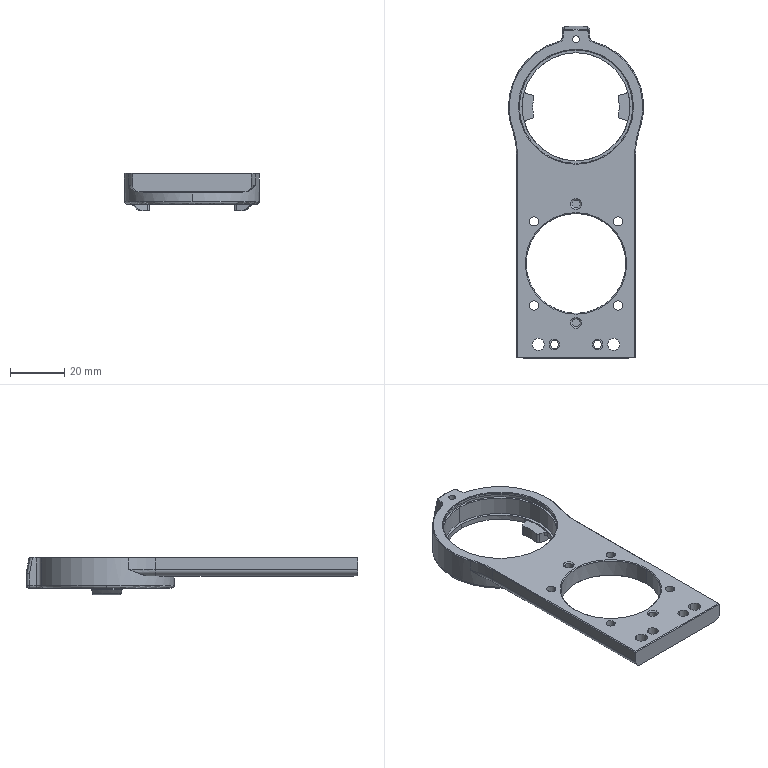NC program | NX | posted with a generic post | part box 50 x 122.9 x 14 mm
Lines 2916 to 3839 of 10876:
(ZLEVEL_PROFILE_1_COPY , TOOL : D3R0.5)
N5782 T18 M6
N5784 G54
N5786 G17 G0 G90 X85.63 Y20.139 S9500 M3
N5788 G43 Z30. H18
N5790 Z2.993
N5792 G94 G1 Z-0.007 F1000.
N5794 G3 X87.271 Y19.45 R1.5
N5796 G1 X87.74 Y19.631 F2500.
N5798 G2 X98.26 Y19.631 R20.323
N5800 G1 X98.73 Y19.453
N5802 X98.762 Y19.571 Z-0.013
N5804 X98.773 Y19.611 Z-0.018
N5806 X98.299 Y19.775
N5808 G3 X87.701 Y19.775 R20.472
N5810 G1 X87.229 Y19.606
N5812 X87.208 Y19.683 Z-0.026
N5814 X87.199 Y19.719 Z-0.033
N5816 X87.674 Y19.876
N5818 G2 X98.326 Y19.876 R20.577
N5820 G1 X98.802 Y19.722
N5822 X98.818 Y19.783 Z-0.043
N5824 X98.827 Y19.816 Z-0.052
N5826 X98.352 Y19.973
N5828 G3 X87.648 Y19.973 R20.678
N5830 G1 X87.173 Y19.816
N5832 X87.156 Y19.879 Z-0.063
N5834 X87.143 Y19.927 Z-0.074
N5836 X87.559 Y20.038
N5838 X87.622 Y20.069
N5840 G2 X98.378 Y20.069 R20.777
N5842 G1 X98.857 Y19.927
N5844 X98.87 Y19.976 Z-0.088
N5846 X98.88 Y20.013 Z-0.101
N5848 X98.403 Y20.164
N5850 G3 X87.597 Y20.164 R20.875
N5852 G1 X87.119 Y20.015
N5854 X87.104 Y20.073 Z-0.116
N5856 X87.093 Y20.113 Z-0.131
N5858 X87.572 Y20.257
N5860 G2 X98.428 Y20.257 R20.971
N5862 G1 X98.906 Y20.111
N5864 X98.92 Y20.162 Z-0.148
N5866 X98.931 Y20.202 Z-0.166
N5868 X98.453 Y20.348
N5870 G3 X87.547 Y20.348 R21.066
N5872 G1 X87.067 Y20.209
N5874 X87.055 Y20.256 Z-0.184
N5876 X87.045 Y20.292 Z-0.203
N5878 X87.523 Y20.438
N5880 G2 X98.477 Y20.438 R21.159
N5882 G1 X98.953 Y20.285
N5884 X98.967 Y20.337 Z-0.224
N5886 X98.977 Y20.375 Z-0.244
N5888 X98.546 Y20.504
N5890 X98.5 Y20.525
N5892 G3 X87.5 Y20.525 R21.25
N5894 G1 X87.021 Y20.383
N5896 X87.009 Y20.428 Z-0.267
N5898 X86.999 Y20.464 Z-0.289
N5900 X87.477 Y20.611
N5902 G2 X98.523 Y20.611 R21.339
N5904 G1 X99.001 Y20.465
N5906 X99.014 Y20.513 Z-0.313
N5908 X99.025 Y20.556 Z-0.338
N5910 X98.302 Y20.76
N5912 G3 X87.454 Y20.696 R21.426
N5914 G1 X87.071 Y20.572
N5916 X86.978 Y20.544
N5918 X86.965 Y20.592 Z-0.363
N5920 X86.955 Y20.631 Z-0.389
N5922 X87.432 Y20.778
N5924 G2 X98.568 Y20.778 R21.511
N5926 G1 X99.048 Y20.641
N5928 X99.059 Y20.683 Z-0.417
N5930 X99.067 Y20.715 Z-0.444
N5932 X98.589 Y20.859
N5934 G3 X87.411 Y20.859 R21.594
N5936 G1 X86.934 Y20.71
N5938 X86.922 Y20.754 Z-0.474
N5940 X86.913 Y20.788 Z-0.503
N5942 X87.39 Y20.937
N5944 G2 X98.61 Y20.937 R21.675
N5946 G1 X99.034 Y20.807
N5948 X99.087 Y20.789
N5950 X99.099 Y20.836 Z-0.534
N5952 X99.107 Y20.867 Z-0.564
N5954 X98.631 Y21.013
N5956 G3 X87.369 Y21.013 R21.754
N5958 G1 X87.315 Y20.989
N5960 X86.891 Y20.87
N5962 X86.881 Y20.909 Z-0.597
N5964 X86.871 Y20.945 Z-0.629
N5966 X87.315 Y21.069
N5968 X87.35 Y21.086
N5970 G2 X98.65 Y21.086 R21.83
N5972 G1 X99.127 Y20.94
N5974 X99.137 Y20.983 Z-0.662
N5976 X99.145 Y21.011 Z-0.696
N5978 X98.669 Y21.156
N5980 G3 X87.331 Y21.156 R21.902
N5982 G1 X86.853 Y21.016
N5984 X86.843 Y21.056 Z-0.73
N5986 X86.834 Y21.09 Z-0.765
N5988 X87.313 Y21.223
N5990 G2 X98.687 Y21.223 R21.972
N5992 G1 X99.163 Y21.084
N5994 X99.174 Y21.125 Z-0.8
N5996 X99.182 Y21.158 Z-0.835
N5998 X98.706 Y21.291
N6000 G3 X87.294 Y21.291 R22.042
N6002 G1 X86.816 Y21.16
N6004 X86.807 Y21.195 Z-0.87
N6006 X86.799 Y21.227 Z-0.906
N6008 X86.827 Y21.236
N6010 X87.276 Y21.359
N6012 G2 X98.724 Y21.359 R22.113
N6014 G1 X99.199 Y21.226
N6016 X99.209 Y21.262 Z-0.941
N6018 X99.217 Y21.295 Z-0.976
N6020 X98.742 Y21.427
N6022 G3 X87.258 Y21.427 R22.184
N6024 G1 X86.827 Y21.31
N6026 X86.782 Y21.295
N6028 X86.773 Y21.332 Z-1.012
N6030 X86.765 Y21.363 Z-1.047
N6032 X86.827 Y21.383
N6034 X87.24 Y21.496
N6036 G2 X98.76 Y21.496 R22.254
N6038 G1 X99.234 Y21.365
N6040 X99.243 Y21.4 Z-1.082
N6042 X99.252 Y21.434 Z-1.118
N6044 X98.779 Y21.564
N6046 G3 X87.221 Y21.564 R22.325
N6048 G1 X86.827 Y21.457
N6050 X86.748 Y21.432
N6052 X86.739 Y21.469 Z-1.153
N6054 X86.731 Y21.5 Z-1.189
N6056 X87.203 Y21.632
N6058 G2 X98.797 Y21.632 R22.396
N6060 G1 X99.269 Y21.503
N6062 X99.278 Y21.537 Z-1.224
N6064 X99.286 Y21.571 Z-1.259
N6066 X98.815 Y21.701
N6068 G3 X87.185 Y21.701 R22.466
N6070 G1 X86.713 Y21.569
N6072 X86.704 Y21.607 Z-1.295
N6074 X86.695 Y21.64 Z-1.33
N6076 X87.166 Y21.769
N6078 G2 X98.834 Y21.769 R22.537
N6080 G1 X99.304 Y21.64
N6082 X99.312 Y21.675 Z-1.365
N6084 X99.32 Y21.706 Z-1.401
N6086 X98.852 Y21.837
N6088 G3 X87.148 Y21.837 R22.608
N6090 G1 X87.071 Y21.817
N6092 X86.679 Y21.708
N6094 X86.669 Y21.744 Z-1.436
N6096 X86.661 Y21.777 Z-1.471
N6098 X87.13 Y21.906
N6100 G2 X98.87 Y21.906 R22.678
N6102 G1 X99.278 Y21.794
N6104 X99.338 Y21.775
N6106 X99.347 Y21.812 Z-1.507
N6108 X99.355 Y21.843 Z-1.542
N6110 X99.278 Y21.868
N6112 X98.889 Y21.974
N6114 G3 X87.111 Y21.974 R22.749
N6116 G1 X86.644 Y21.846
N6118 X86.635 Y21.882 Z-1.577
N6120 X86.626 Y21.915 Z-1.613
N6122 X87.093 Y22.042
N6124 G2 X98.907 Y22.042 R22.82
N6126 G1 X99.372 Y21.913
N6128 X99.382 Y21.95 Z-1.648
N6130 X99.39 Y21.981 Z-1.684
N6132 X98.925 Y22.11
N6134 G3 X87.075 Y22.11 R22.891
N6136 G1 X86.609 Y21.984
N6138 X86.6 Y22.019 Z-1.719
N6140 X86.592 Y22.053 Z-1.754
N6142 X87.057 Y22.179
N6144 G2 X98.943 Y22.179 R22.961
N6146 G1 X99.407 Y22.05
N6148 X99.416 Y22.088 Z-1.79
N6150 X99.425 Y22.122 Z-1.825
N6152 X98.962 Y22.247
N6154 G3 X87.038 Y22.247 R23.032
N6156 G1 X86.574 Y22.122
N6158 X86.566 Y22.157 Z-1.86
N6160 X86.558 Y22.189 Z-1.896
N6162 X86.583 Y22.198
N6164 X87.02 Y22.315
N6166 G2 X98.98 Y22.315 R23.103
N6168 G1 X99.442 Y22.189
N6170 X99.451 Y22.225 Z-1.931
N6172 X99.459 Y22.258 Z-1.966
N6174 X98.998 Y22.384
N6176 G3 X87.002 Y22.384 R23.173
N6178 G1 X86.583 Y22.271
N6180 X86.541 Y22.257
N6182 X86.531 Y22.294 Z-2.002
N6184 X86.524 Y22.325 Z-2.037
N6186 X86.583 Y22.344
N6188 X86.983 Y22.452
N6190 G2 X99.017 Y22.452 R23.244
N6192 G1 X99.477 Y22.328
N6194 X99.486 Y22.363 Z-2.072
N6196 X99.494 Y22.397 Z-2.108
N6198 X98.862 Y22.566
N6200 G3 X86.965 Y22.52 R23.315
N6202 G1 X86.583 Y22.418
N6204 X86.5 Y22.393
N6206 X86.461 Y22.453 Z-2.178
N6208 G2 X99.512 Y22.466 R23.498
N6210 G1 X99.579 Y22.482 Z-2.214
N6212 X99.644 Y22.491 Z-2.249
N6214 G3 X86.461 Y22.528 R23.48
N6216 G1 X86.413 Y22.589 Z-2.32
N6218 G2 X99.644 Y22.566 R23.652
N6220 G1 X99.608 Y22.621 Z-2.355
N6222 X99.57 Y22.669 Z-2.391
N6224 G3 X86.441 Y22.673 R23.907
N6226 G1 X86.431 Y22.707 Z-2.426
N6228 X86.422 Y22.741 Z-2.461
N6230 G2 X99.577 Y22.741 R23.904
N6232 G3 X101.28 Y23.418 R1.5
N6234 G1 Z0.539
N6236 G0 Z30.
N6238 X100.348 Y-20.179
N6240 Z2.993
N6242 G1 Z-0.007 F1000.
N6244 G3 X98.73 Y-19.452 R1.5
N6246 G1 X98.26 Y-19.631 F2500.
N6248 G2 X87.74 Y-19.631 R20.323
N6250 G1 X87.27 Y-19.451
N6252 X87.242 Y-19.556 Z-0.013
N6254 X87.229 Y-19.607 Z-0.018
N6256 X87.701 Y-19.775
N6258 G3 X98.299 Y-19.775 R20.472
N6260 G1 X98.772 Y-19.61
N6262 X98.792 Y-19.685 Z-0.026
N6264 X98.802 Y-19.722 Z-0.033
N6266 X98.326 Y-19.876
N6268 G2 X87.674 Y-19.876 R20.577
N6270 G1 X87.199 Y-19.719
N6272 X87.182 Y-19.783 Z-0.043
N6274 X87.173 Y-19.816 Z-0.052
N6276 X87.648 Y-19.973
N6278 G3 X98.352 Y-19.973 R20.678
N6280 G1 X98.827 Y-19.815
N6282 X98.844 Y-19.879 Z-0.063
N6284 X98.857 Y-19.927 Z-0.074
N6286 X98.378 Y-20.069
N6288 G2 X87.622 Y-20.069 R20.777
N6290 G1 X87.559 Y-20.038
N6292 X87.143 Y-19.928
N6294 X87.13 Y-19.976 Z-0.088
N6296 X87.12 Y-20.015 Z-0.101
N6298 X87.597 Y-20.164
N6300 G3 X98.403 Y-20.164 R20.875
N6302 G1 X98.88 Y-20.013
N6304 X98.896 Y-20.073 Z-0.116
N6306 X98.906 Y-20.112 Z-0.131
N6308 X98.428 Y-20.257
N6310 G2 X87.572 Y-20.257 R20.971
N6312 G1 X87.093 Y-20.112
N6314 X87.08 Y-20.162 Z-0.148
N6316 X87.068 Y-20.206 Z-0.166
N6318 X87.547 Y-20.348
N6320 G3 X98.453 Y-20.348 R21.066
N6322 G1 X98.931 Y-20.205
N6324 X98.945 Y-20.256 Z-0.184
N6326 X98.955 Y-20.292 Z-0.203
N6328 X98.477 Y-20.438
N6330 G2 X87.523 Y-20.438 R21.159
N6332 G1 X87.447 Y-20.412
N6334 X87.047 Y-20.286
N6336 X87.033 Y-20.337 Z-0.224
N6338 X87.024 Y-20.373 Z-0.244
N6340 X87.5 Y-20.525
N6342 G3 X98.5 Y-20.525 R21.25
N6344 G1 X98.546 Y-20.504
N6346 X98.98 Y-20.386
N6348 X98.991 Y-20.428 Z-0.267
N6350 X99.002 Y-20.468 Z-0.289
N6352 X98.523 Y-20.611
N6354 G2 X87.477 Y-20.611 R21.339
N6356 G1 X87. Y-20.46
N6358 X86.986 Y-20.514 Z-0.313
N6360 X86.977 Y-20.547 Z-0.338
N6362 X87.454 Y-20.696
N6364 G3 X98.302 Y-20.76 R21.426
N6366 X99.024 Y-20.549 R11.109
N6368 G1 X99.035 Y-20.592 Z-0.363
N6370 X99.046 Y-20.633 Z-0.389
N6372 X98.568 Y-20.778
N6374 G2 X87.432 Y-20.778 R21.511
N6376 G1 X86.952 Y-20.64
N6378 X86.941 Y-20.683 Z-0.417
N6380 X86.932 Y-20.716 Z-0.444
N6382 X87.411 Y-20.859
N6384 G3 X98.589 Y-20.859 R21.594
N6386 G1 X99.066 Y-20.709
N6388 X99.078 Y-20.754 Z-0.474
N6390 X99.086 Y-20.786 Z-0.503
N6392 X98.61 Y-20.937
N6394 G2 X87.39 Y-20.937 R21.675
N6396 G1 X86.912 Y-20.792
N6398 X86.901 Y-20.836 Z-0.534
N6400 X86.892 Y-20.87 Z-0.564
N6402 X87.315 Y-20.989
N6404 X87.369 Y-21.013
N6406 G3 X98.631 Y-21.013 R21.754
N6408 G1 X99.108 Y-20.867
N6410 X99.119 Y-20.91 Z-0.597
N6412 X99.128 Y-20.942 Z-0.629
N6414 X98.65 Y-21.086
N6416 G2 X87.35 Y-21.086 R21.83
N6418 G1 X86.873 Y-20.943
N6420 X86.863 Y-20.982 Z-0.662
N6422 X86.854 Y-21.014 Z-0.696
N6424 X87.331 Y-21.156
N6426 G3 X98.669 Y-21.156 R21.902
N6428 G1 X99.146 Y-21.013
N6430 X99.157 Y-21.056 Z-0.73
N6432 X99.165 Y-21.086 Z-0.765
N6434 X98.687 Y-21.223
N6436 G2 X87.313 Y-21.223 R21.972
N6438 G1 X86.835 Y-21.088
N6440 X86.826 Y-21.125 Z-0.8
N6442 X86.817 Y-21.158 Z-0.835
N6444 X87.295 Y-21.291
N6446 G3 X98.705 Y-21.291 R22.042
N6448 G1 X99.184 Y-21.159
N6450 X99.193 Y-21.195 Z-0.87
N6452 X99.201 Y-21.227 Z-0.906
N6454 X98.724 Y-21.359
N6456 G2 X87.276 Y-21.359 R22.113
N6458 G1 X86.801 Y-21.226
N6460 X86.792 Y-21.262 Z-0.941
N6462 X86.784 Y-21.294 Z-0.976
N6464 X87.258 Y-21.428
N6466 G3 X98.742 Y-21.428 R22.184
N6468 G1 X99.218 Y-21.296
N6470 X99.227 Y-21.332 Z-1.012
N6472 X99.236 Y-21.366 Z-1.047
N6474 X98.76 Y-21.496
N6476 G2 X87.24 Y-21.496 R22.254
N6478 G1 X86.827 Y-21.382
N6480 X86.766 Y-21.362
N6482 X86.757 Y-21.4 Z-1.082
N6484 X86.749 Y-21.431 Z-1.118
N6486 X87.221 Y-21.564
N6488 G3 X98.779 Y-21.564 R22.325
N6490 G1 X99.253 Y-21.435
N6492 X99.262 Y-21.469 Z-1.153
N6494 X99.27 Y-21.504 Z-1.189
N6496 X98.797 Y-21.632
N6498 G2 X87.203 Y-21.632 R22.396
N6500 G1 X86.732 Y-21.499
N6502 X86.722 Y-21.537 Z-1.224
N6504 X86.714 Y-21.568 Z-1.259
N6506 X87.185 Y-21.701
N6508 G3 X98.815 Y-21.701 R22.466
N6510 G1 X99.287 Y-21.572
N6512 X99.296 Y-21.607 Z-1.295
N6514 X99.305 Y-21.64 Z-1.33
N6516 X98.833 Y-21.769
N6518 G2 X87.167 Y-21.769 R22.537
N6520 G1 X86.696 Y-21.64
N6522 X86.687 Y-21.675 Z-1.365
N6524 X86.679 Y-21.707 Z-1.401
N6526 X87.148 Y-21.837
N6528 G3 X98.852 Y-21.837 R22.608
N6530 G1 X99.278 Y-21.722
N6532 X99.321 Y-21.707
N6534 X99.33 Y-21.744 Z-1.436
N6536 X99.338 Y-21.775 Z-1.471
N6538 X99.278 Y-21.795
N6540 X98.87 Y-21.906
N6542 G2 X87.13 Y-21.906 R22.678
N6544 G1 X86.662 Y-21.776
N6546 X86.653 Y-21.812 Z-1.507
N6548 X86.644 Y-21.846 Z-1.542
N6550 X87.112 Y-21.974
N6552 G3 X98.888 Y-21.974 R22.749
N6554 G1 X99.278 Y-21.869
N6556 X99.356 Y-21.844
N6558 X99.365 Y-21.882 Z-1.577
N6560 X99.373 Y-21.913 Z-1.613
N6562 X98.907 Y-22.042
N6564 G2 X87.093 Y-22.042 R22.82
N6566 G1 X86.627 Y-21.915
N6568 X86.618 Y-21.95 Z-1.648
N6570 X86.609 Y-21.984 Z-1.684
N6572 X87.075 Y-22.111
N6574 G3 X98.925 Y-22.111 R22.891
N6576 G1 X99.39 Y-21.982
N6578 X99.4 Y-22.019 Z-1.719
N6580 X99.408 Y-22.051 Z-1.754
N6582 X98.943 Y-22.179
N6584 G2 X87.057 Y-22.179 R22.961
N6586 G1 X86.592 Y-22.053
N6588 X86.583 Y-22.087 Z-1.79
N6590 X86.575 Y-22.122 Z-1.825
N6592 X87.038 Y-22.247
N6594 G3 X98.962 Y-22.247 R23.032
N6596 G1 X99.426 Y-22.122
N6598 X99.434 Y-22.157 Z-1.86
N6600 X99.443 Y-22.189 Z-1.896
N6602 X98.98 Y-22.315
N6604 G2 X87.02 Y-22.315 R23.103
N6606 G1 X86.583 Y-22.197
N6608 X86.558 Y-22.189
N6610 X86.549 Y-22.225 Z-1.931
N6612 X86.541 Y-22.257 Z-1.966
N6614 X86.583 Y-22.271
N6616 X87.002 Y-22.384
N6618 G3 X98.998 Y-22.384 R23.173
N6620 G1 X99.46 Y-22.258
N6622 X99.469 Y-22.294 Z-2.002
N6624 X99.477 Y-22.328 Z-2.037
N6626 X99.016 Y-22.452
N6628 G2 X86.984 Y-22.452 R23.244
N6630 G1 X86.583 Y-22.344
N6632 X86.524 Y-22.325
N6634 X86.514 Y-22.363 Z-2.072
N6636 X86.506 Y-22.394 Z-2.108
N6638 X86.583 Y-22.418
N6640 X86.965 Y-22.52
N6642 G3 X98.861 Y-22.566 R23.315
N6644 G1 X99.495 Y-22.397
N6646 X99.503 Y-22.431 Z-2.143
N6648 X99.512 Y-22.466 Z-2.178
N6650 G2 X86.49 Y-22.462 R23.513
N6652 G1 X86.48 Y-22.5 Z-2.214
N6654 X86.472 Y-22.531 Z-2.249
N6656 G3 X99.644 Y-22.491 R23.549
N6658 G1 Y-22.566 Z-2.32
N6660 G2 X87.071 Y-22.762 R23.504
N6662 G1 X86.487 Y-22.612
N6664 X86.455 Y-22.602
N6666 X86.504 Y-22.688 Z-2.391
N6668 G3 X90.489 Y-23.462 R25.369
N6670 X99.57 Y-22.67 R24.129
N6672 G1 X99.573 Y-22.706 Z-2.426
N6674 X99.577 Y-22.741 Z-2.461
N6676 G2 X86.563 Y-22.777 R24.031
N6678 G3 X84.832 Y-23.527 R1.5
N6680 G1 Z0.539
N6682 G0 Z30.
N6684 X118.849 Y-6.691
N6686 Z0.495
N6688 G1 Z-2.505 F1000.
N6690 Y-6.616
N6692 G2 X120.349 Y-5.116 R1.5
N6694 G1 X121.622 F2500.
N6696 G3 X122.727 Y-4.155 R1.116
N6698 X122.727 Y4.155 R30.016
N6700 X121.622 Y5.116 R1.116
N6702 G1 X119.077
N6704 G2 X117.257 Y6.512 R1.884
N6706 G3 X117.257 Y-6.512 R-25.116
N6708 G2 X119.077 Y-5.116 R1.884
N6710 G1 X120.349
N6712 Y-5.188 Z-2.512
N6714 Y-5.24 Z-2.519
N6716 X119.077
N6718 G3 X117.377 Y-6.544 R1.76
N6720 G2 X117.377 Y6.544 R-25.24
N6722 G3 X119.077 Y5.24 R1.76
N6724 G1 X121.622
N6726 G2 X122.849 Y4.172 R1.24
N6728 X122.849 Y-4.172 R30.14
N6730 X121.622 Y-5.24 R1.24
N6732 G1 X120.349
N6734 Y-5.297 Z-2.53
N6736 Y-5.345 Z-2.54
N6738 X121.622
N6740 G3 X122.954 Y-4.186 R1.345
N6742 X122.954 Y4.186 R30.245
N6744 X121.622 Y5.345 R1.345
N6746 G1 X119.077
N6748 G2 X117.479 Y6.571 R1.655
N6750 G3 X117.479 Y-6.571 R-25.345
N6752 G2 X119.077 Y-5.345 R1.655
N6754 G1 X120.349
N6756 Y-5.399 Z-2.554
N6758 Y-5.446 Z-2.568
N6760 X119.077
N6762 G3 X117.576 Y-6.597 R1.554
N6764 G2 X117.576 Y6.597 R-25.446
N6766 G3 X119.077 Y5.446 R1.554
N6768 G1 X121.622
N6770 G2 X123.054 Y4.2 R1.446
N6772 X123.054 Y-4.2 R30.346
N6774 X121.622 Y-5.446 R1.446
N6776 G1 X120.349
N6778 Y-5.497 Z-2.585
N6780 Y-5.543 Z-2.602
N6782 X121.622
N6784 G3 X123.15 Y-4.214 R1.543
N6786 X123.15 Y4.214 R30.443
N6788 X121.622 Y5.543 R1.543
N6790 G1 X119.077
N6792 G2 X117.669 Y6.622 R1.457
N6794 G3 X117.669 Y-6.622 R-25.543
N6796 G2 X119.077 Y-5.543 R1.457
N6798 G1 X120.349
N6800 Y-5.592 Z-2.622
N6802 Y-5.637 Z-2.642
N6804 X119.077
N6806 G3 X117.76 Y-6.647 R1.363
N6808 G2 X117.76 Y6.647 R-25.637
N6810 G3 X119.077 Y5.637 R1.363
N6812 G1 X121.622
N6814 G2 X123.243 Y4.227 R1.637
N6816 X123.243 Y-4.227 R30.537
N6818 X121.622 Y-5.637 R1.637
N6820 G1 X120.349
N6822 Y-5.684 Z-2.665
N6824 Y-5.727 Z-2.688
N6826 X121.622
N6828 G3 X123.332 Y-4.239 R1.727
N6830 X123.332 Y4.239 R30.627
N6832 X121.622 Y5.727 R1.727
N6834 G1 X119.077
N6836 G2 X117.847 Y6.67 R1.273
N6838 G3 X117.847 Y-6.67 R-25.727
N6840 G2 X119.077 Y-5.727 R1.273
N6842 G1 X120.349
N6844 Y-5.772 Z-2.714
N6846 Y-5.814 Z-2.74
N6848 X119.077
N6850 G3 X117.931 Y-6.692 R1.186
N6852 G2 X117.931 Y6.692 R-25.814
N6854 G3 X119.077 Y5.814 R1.186
N6856 G1 X121.622
N6858 G2 X123.418 Y4.251 R1.814
N6860 X123.418 Y-4.251 R30.714
N6862 X121.622 Y-5.814 R1.814
N6864 G1 X120.349
N6866 Y-5.856 Z-2.769
N6868 Y-5.896 Z-2.797
N6870 X121.622
N6872 G3 X123.5 Y-4.262 R1.896
N6874 X123.5 Y4.262 R30.796
N6876 X121.622 Y5.896 R1.896
N6878 G1 X119.077
N6880 G2 X118.011 Y6.714 R1.104
N6882 G3 X118.011 Y-6.714 R-25.896
N6884 G2 X119.077 Y-5.896 R1.104
N6886 G1 X120.349
N6888 Y-5.937 Z-2.829
N6890 Y-5.975 Z-2.86
N6892 X119.077
N6894 G3 X118.087 Y-6.734 R1.025
N6896 G2 X118.087 Y6.734 R-25.975
N6898 G3 X119.077 Y5.975 R1.025
N6900 G1 X121.622
N6902 G2 X123.578 Y4.273 R1.975
N6904 X123.578 Y-4.273 R30.875
N6906 X121.622 Y-5.975 R1.975
N6908 G1 X120.349
N6910 Y-6.013 Z-2.894
N6912 Y-6.049 Z-2.928
N6914 X121.622
N6916 G3 X123.651 Y-4.284 R2.049
N6918 X123.651 Y4.284 R30.949
N6920 X121.622 Y6.049 R2.049
N6922 G1 X119.077
N6924 G2 X118.159 Y6.753 R0.951
N6926 G3 X118.159 Y-6.753 R-26.049
N6928 G2 X119.077 Y-6.049 R0.951
N6930 G1 X120.349
N6932 Y-6.085 Z-2.964
N6934 Y-6.119 Z-3.001
N6936 X119.077
N6938 G3 X118.226 Y-6.771 R0.881
N6940 G2 X118.226 Y6.771 R-26.119
N6942 G3 X119.077 Y6.119 R0.881
N6944 G1 X121.622
N6946 G2 X123.72 Y4.293 R2.119
N6948 X123.72 Y-4.293 R31.019
N6950 X121.622 Y-6.119 R2.119
N6952 G1 X120.349
N6954 Y-6.152 Z-3.039
N6956 Y-6.183 Z-3.078
N6958 X121.622
N6960 G3 X123.784 Y-4.302 R2.183
N6962 X123.784 Y4.302 R31.083
N6964 X121.622 Y6.183 R2.183
N6966 G1 X119.077
N6968 G2 X118.288 Y6.788 R0.817
N6970 G3 X118.288 Y-6.788 R-26.183
N6972 G2 X119.077 Y-6.183 R0.817
N6974 G1 X120.349
N6976 Y-6.213 Z-3.118
N6978 Y-6.242 Z-3.159
N6980 X119.077
N6982 G3 X118.345 Y-6.803 R0.758
N6984 G2 X118.345 Y6.803 R-26.242
N6986 G3 X119.077 Y6.242 R0.758
N6988 G1 X121.622
N6990 G2 X123.842 Y4.31 R2.242
N6992 X123.842 Y-4.31 R31.142
N6994 X121.622 Y-6.242 R2.242
N6996 G1 X120.349
N6998 Y-6.27 Z-3.201
N7000 Y-6.295 Z-3.244
N7002 X121.622
N7004 G3 X123.895 Y-4.318 R2.295
N7006 X123.895 Y4.318 R31.195
N7008 X121.622 Y6.295 R2.295
N7010 G1 X119.077
N7012 G2 X118.396 Y6.817 R0.705
N7014 G3 X118.396 Y-6.817 R-26.295
N7016 G2 X119.077 Y-6.295 R0.705
N7018 G1 X120.349
N7020 Y-6.32 Z-3.288
N7022 Y-6.343 Z-3.332
N7024 X119.077
N7026 G3 X118.442 Y-6.83 R0.657
N7028 G2 X118.442 Y6.83 R-26.343
N7030 G3 X119.077 Y6.343 R0.657
N7032 G1 X121.622
N7034 G2 X123.942 Y4.324 R2.343
N7036 X123.942 Y-4.324 R31.243
N7038 X121.622 Y-6.343 R2.343
N7040 G1 X120.349
N7042 Y-6.365 Z-3.377
N7044 Y-6.384 Z-3.423
N7046 X121.622
N7048 G3 X123.983 Y-4.33 R2.384
N7050 X123.983 Y4.33 R31.284
N7052 X121.622 Y6.384 R2.384
N7054 G1 X119.077
N7056 G2 X118.482 Y6.84 R0.616
N7058 G3 X118.482 Y-6.84 R-26.384
N7060 G2 X119.077 Y-6.384 R0.616
N7062 G1 X120.349
N7064 Y-6.403 Z-3.47
N7066 Y-6.42 Z-3.516
N7068 X119.077
N7070 G3 X118.517 Y-6.85 R0.58
N7072 G2 X118.517 Y6.85 R-26.42
N7074 G3 X119.077 Y6.42 R0.58
N7076 G1 X121.622
N7078 G2 X124.018 Y4.335 R2.42
N7080 X124.018 Y-4.335 R31.32
N7082 X121.622 Y-6.42 R2.42
N7084 G1 X120.349
N7086 Y-6.435 Z-3.564
N7088 Y-6.449 Z-3.612
N7090 X121.622
N7092 G3 X124.047 Y-4.339 R2.449
N7094 X124.047 Y4.339 R31.349
N7096 X121.622 Y6.449 R2.449
N7098 G1 X119.077
N7100 G2 X118.545 Y6.857 R0.551
N7102 G3 X118.545 Y-6.857 R-26.449
N7104 G2 X119.077 Y-6.449 R0.551
N7106 G1 X120.349
N7108 Y-6.461 Z-3.661
N7110 Y-6.472 Z-3.709
N7112 X119.077
N7114 G3 X118.566 Y-6.863 R0.528
N7116 G2 X118.566 Y6.863 R-26.472
N7118 G3 X119.077 Y6.472 R0.528
N7120 G1 X121.622
N7122 G2 X124.07 Y4.342 R2.472
N7124 X124.07 Y-4.342 R31.372
N7126 X121.622 Y-6.472 R2.472
N7128 G1 X120.349
N7130 Y-6.48 Z-3.758
N7132 Y-6.487 Z-3.806
N7134 X121.622
N7136 G3 X124.085 Y-4.344 R2.487
N7138 X124.085 Y4.344 R31.387
N7140 X121.622 Y6.487 R2.487
N7142 G1 X119.077
N7144 G2 X118.582 Y6.867 R0.513
N7146 G3 X118.582 Y-6.867 R-26.487
N7148 G2 X119.077 Y-6.487 R0.513
N7150 G1 X120.349
N7152 Y-6.497 Z-3.903
N7154 X119.077
N7156 G3 X118.591 Y-6.87 R0.503
N7158 G2 X97.081 Y26.181 R-26.497
N7160 G1 X97.325 Y26.141
N7162 G2 X118.591 Y6.87 R26.497
N7164 G3 X119.077 Y6.497 R0.503
N7166 G1 X121.622
N7168 G2 X124.095 Y4.346 R2.497
N7170 X124.095 Y-4.346 R31.397
N7172 X121.622 Y-6.497 R2.497
N7174 G1 X120.349
N7176 Y-6.5 Z-4.
N7178 X121.622
N7180 G3 X124.097 Y-4.346 R2.501
N7182 X124.097 Y4.346 R31.526
N7184 X121.984 Y6.471 R2.497
N7186 G1 X121.622 Y6.5
N7188 X121.495 Y6.498
N7190 X119.298 Y6.5
N7192 X119.077
N7194 G2 X118.808 Y6.579 R0.5
N7196 X118.594 Y6.87 R0.5
N7198 G3 X114.904 Y14.915 R26.5
N7200 X97.325 Y26.141 R26.518
N7202 X89.024 Y26.197 R26.392
N7204 X113.683 Y-16.567 R-26.499
N7206 X118.594 Y-6.87 R26.5
N7208 G2 X119.077 Y-6.5 R0.5
N7210 G1 X119.298
N7212 X120.349
N7214 G2 X121.85 Y-7.993 R1.5
N7216 G1 Z-1.
N7218 G0 Z30.
(ZLEVEL_PROFILE_1_COPY_COPY , TOOL : D3R0.5)
N7220 X87.592 Y-27.471
N7222 Z-0.5
N7224 G1 Z-3.5 F1000.
N7226 G3 X86.493 Y-25.687 R1.5
N7228 G2 X85.133 Y-25.302 R22.965 F2500.
N7230 G1 X84.792 Y-25.188
N7232 X84.775 Y-25.187
N7234 X84.373 Y-25.056
N7236 X84.368 Y-25.053
N7238 X84.22 Y-24.992
N7240 X83.605 Y-24.776
N7242 X83.549 Y-24.756
N7244 X83.536 Y-24.752
N7246 X82.93 Y-24.512
N7248 X82.907 Y-24.493
N7250 X82.729 Y-24.421
N7252 X82.402 Y-24.284
N7254 X82.393 Y-24.283
N7256 X82.326 Y-24.255
N7258 X82.101 Y-24.155
N7260 X82.085 Y-24.141
N7262 X81.967 Y-24.089
N7264 X81.938 Y-24.079
N7266 X81.818 Y-24.024
N7268 X81.807 Y-24.02
N7270 X81.511 Y-23.88
N7272 X81.509 Y-23.876
N7274 X81.253 Y-23.744
N7276 X81.238 Y-23.747
N7278 X80.939 Y-23.596
N7280 X80.904 Y-23.576
N7282 X80.794 Y-23.519
N7284 X80.775 Y-23.504
N7286 X80.673 Y-23.449
N7288 X80.661 Y-23.452
N7290 X79.854 Y-23.009
N7292 X79.842 Y-22.995
N7294 X79.248 Y-22.646
N7296 X79.085 Y-22.553
N7298 X78.963 Y-22.477
N7300 X78.951 Y-22.46
N7302 X78.82 Y-22.378
N7304 X78.8 Y-22.367
N7306 X78.419 Y-22.123
N7308 X78.41 Y-22.12
N7310 X78.333 Y-22.07
N7312 X78.09 Y-21.907
N7314 X78.089 Y-21.902
N7316 X78.027 Y-21.856
N7318 X78.01 Y-21.853
N7320 X77.934 Y-21.799
N7322 X77.92 Y-21.791
N7324 X77.688 Y-21.628
N7326 X77.629 Y-21.586
N7328 X77.605 Y-21.568
N7330 X77.355 Y-21.379
N7332 X77.34 Y-21.378
N7334 X77.111 Y-21.209
N7336 Y-21.205
N7338 X76.866 Y-21.016
N7340 X76.831 Y-20.985
N7342 X76.816 Y-20.984
N7344 X76.442 Y-20.69
N7346 X76.418 Y-20.649
N7348 X76.373 Y-20.631
N7350 X76.369
N7352 X75.99 Y-20.313
N7354 X75.48 Y-19.882
N7356 X75.373 Y-19.787
N7358 X75.371 Y-19.762
N7360 X75.348 Y-19.751
N7362 G2 X74.824 Y-19.271 R7.352
N7364 G1 X74.794 Y-19.256
N7366 X74.724 Y-19.19
N7368 X74.223 Y-18.7
N7370 X74.183 Y-18.659
N7372 X74.179 Y-18.65
N7374 X73.932 Y-18.399
N7376 X73.929 Y-18.4
N7378 X73.693 Y-18.149
N7380 X73.692 Y-18.146
N7382 X73.446 Y-17.879
N7384 X73.436 Y-17.874
N7386 X73.294 Y-17.718
N7388 X73.267 Y-17.688
N7390 X73.22 Y-17.633
N7392 X73.202 Y-17.607
N7394 X73.085 Y-17.478
N7396 X73.076 Y-17.473
N7398 X72.994 Y-17.377
N7400 X72.981 Y-17.363
N7402 X72.892 Y-17.26
N7404 X72.878 Y-17.234
N7406 X72.84 Y-17.19
N7408 G2 X71.801 Y-15.889 R23.53
N7410 G1 X71.79 Y-15.886
N7412 X71.771 Y-15.859
N7414 Y-15.853
N7416 X71.746 Y-15.828
N7418 X71.675 Y-15.731
N7420 X71.609 Y-15.643
N7422 X71.608 Y-15.631
N7424 X71.558 Y-15.56
N7426 X71.542 Y-15.551
N7428 X71.507 Y-15.502
N7430 X71.384 Y-15.33
N7432 X71.382 Y-15.312
N7434 G2 X71.05 Y-14.83 R8.979
N7436 G1 X71.032 Y-14.82
N7438 X70.868 Y-14.575
N7440 X70.866 Y-14.556
N7442 X70.695 Y-14.3
N7444 X70.686 Y-14.295
N7446 X70.519 Y-14.031
N7448 Y-14.019
N7450 X70.387 Y-13.812
N7452 X70.378 Y-13.784
N7454 X70.363 Y-13.777
N7456 X70.328 Y-13.718
N7458 X70.32 Y-13.707
N7460 X70.182 Y-13.476
N7462 X70.179 Y-13.458
N7464 X70.024 Y-13.199
N7466 X70.021
N7468 X69.79 Y-12.788
N7470 X69.775 Y-12.761
N7472 X69.756 Y-12.726
N7474 X69.585 Y-12.41
N7476 X69.587 Y-12.393
N7478 X69.538 Y-12.31
N7480 X69.214 Y-11.665
N7482 X69.2 Y-11.654
N7484 X69.117 Y-11.482
N7486 Y-11.464
N7488 X69.049 Y-11.331
N7490 X68.842 Y-10.878
N7492 X68.799 Y-10.796
N7494 X68.674 Y-10.512
N7496 X68.676 Y-10.493
N7498 X68.625 Y-10.378
N7500 X68.614 Y-10.372
N7502 X68.45 Y-9.978
N7504 X68.451 Y-9.96
N7506 X68.349 Y-9.709
N7508 Y-9.7
N7510 X68.34 Y-9.702
N7512 X68.319 Y-9.648
N7514 X68.326 Y-9.624
N7516 X68.305 Y-9.612
N7518 X68.216 Y-9.381
N7520 X68.213 Y-9.348
N7522 X68.072 Y-8.982
N7524 X68.065 Y-8.972
N7526 X67.797 Y-8.189
N7528 X67.799 Y-8.185
N7530 X67.8 Y-8.172
N7532 X67.583 Y-7.486
N7534 X67.577 Y-7.477
N7536 X67.526 Y-7.303
N7538 Y-7.271
N7540 X67.342 Y-6.607
N7542 X67.339 Y-6.602
N7544 X67.346 Y-6.559
N7546 X67.316 Y-6.527
N7548 X67.304 Y-6.478
N7550 X67.187 Y-5.995
N7552 X67.189 Y-5.992
N7554 X67.188 Y-5.986
N7556 X67.184 Y-5.984
N7558 X67.105 Y-5.628
N7560 X67.11 Y-5.616
N7562 X67.095 Y-5.571
N7564 X67.056 Y-5.361
N7566 X67.045 Y-5.348
N7568 X66.975 Y-4.996
N7570 X66.979 Y-4.98
N7572 X66.917 Y-4.644
N7574 X66.908 Y-4.63
N7576 X66.851 Y-4.297
N7578 X66.85 Y-4.278
N7580 X66.825 Y-4.094
N7582 X66.816 Y-4.079
N7584 X66.772 Y-3.784
N7586 X66.775 Y-3.785
N7588 X66.778 Y-3.783
N7590 X66.777 Y-3.779
N7592 X66.691 Y-3.1
N7594 X66.68 Y-3.086
N7596 X66.658 Y-2.888
N7598 Y-2.811
N7600 G2 X66.588 Y-2.062 R17.949
N7602 G1 X66.579 Y-2.047
N7604 X66.536 Y-1.375
N7606 X66.542
N7608 X66.541 Y-1.369
N7610 X66.519 Y-0.779
N7612 X66.511 Y-0.764
N7614 X66.504 Y-0.474
N7616 X66.51 Y-0.458